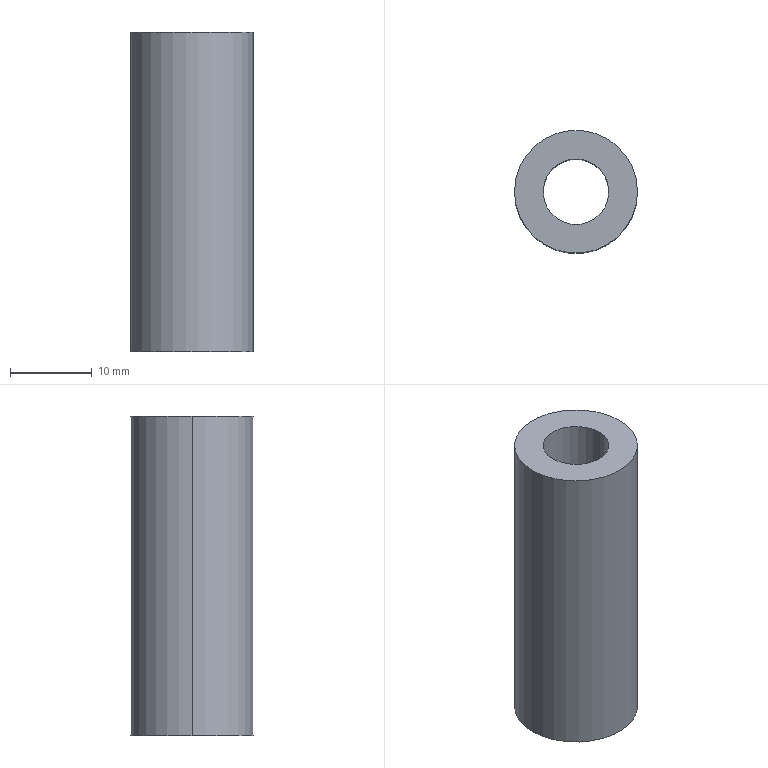Part | SolidWorks | features Extrusion 1 | 1 solid | 6 faces | box 15 x 15 x 39 mm | volume 4932 mm3 | cylinder 4 | plane 2 | commonest cylinder face diameters 8 x2 15 x2
STEP:
#1=CARTESIAN_POINT('',(-4.,0.,39.));
#2=VERTEX_POINT('',#1);
#3=CARTESIAN_POINT('',(4.,0.,39.));
#4=VERTEX_POINT('',#3);
#5=CARTESIAN_POINT('',(0.,0.,39.));
#6=DIRECTION('',(0.,0.,1.));
#7=DIRECTION('',(1.,0.,0.));
#8=AXIS2_PLACEMENT_3D('',#5,#6,#7);
#9=CIRCLE('',#8,4.);
#10=EDGE_CURVE('',#2,#4,#9,.T.);
#11=ORIENTED_EDGE('',*,*,#10,.T.);
#12=CARTESIAN_POINT('',(4.,0.,0.));
#13=VERTEX_POINT('',#12);
#14=CARTESIAN_POINT('',(4.,0.,39.));
#15=DIRECTION('',(0.,0.,-1.));
#16=VECTOR('',#15,1000.);
#17=LINE('',#14,#16);
#18=EDGE_CURVE('',#4,#13,#17,.T.);
#19=ORIENTED_EDGE('',*,*,#18,.T.);
#20=CARTESIAN_POINT('',(-4.,0.,0.));
#21=VERTEX_POINT('',#20);
#22=CARTESIAN_POINT('',(0.,0.,0.));
#23=DIRECTION('',(0.,0.,1.));
#24=DIRECTION('',(1.,0.,0.));
#25=AXIS2_PLACEMENT_3D('',#22,#23,#24);
#26=CIRCLE('',#25,4.);
#27=EDGE_CURVE('',#21,#13,#26,.T.);
#28=ORIENTED_EDGE('',*,*,#27,.F.);
#29=CARTESIAN_POINT('',(-4.,0.,39.));
#30=DIRECTION('',(0.,0.,-1.));
#31=VECTOR('',#30,1000.);
#32=LINE('',#29,#31);
#33=EDGE_CURVE('',#2,#21,#32,.T.);
#34=ORIENTED_EDGE('',*,*,#33,.F.);
#35=EDGE_LOOP('',(#11,#19,#28,#34));
#36=FACE_OUTER_BOUND('',#35,.T.);
#37=CARTESIAN_POINT('',(0.,0.,39.));
#38=DIRECTION('',(0.,0.,-1.));
#39=DIRECTION('',(-1.,0.,0.));
#40=AXIS2_PLACEMENT_3D('',#37,#38,#39);
#41=CYLINDRICAL_SURFACE('',#40,4.);
#42=ADVANCED_FACE('',(#36),#41,.F.);
#43=CARTESIAN_POINT('',(7.5,0.,39.));
#44=VERTEX_POINT('',#43);
#45=CARTESIAN_POINT('',(-7.5,0.,39.));
#46=VERTEX_POINT('',#45);
#47=CARTESIAN_POINT('',(0.,0.,39.));
#48=DIRECTION('',(0.,0.,1.));
#49=DIRECTION('',(1.,0.,0.));
#50=AXIS2_PLACEMENT_3D('',#47,#48,#49);
#51=CIRCLE('',#50,7.5);
#52=EDGE_CURVE('',#44,#46,#51,.T.);
#53=ORIENTED_EDGE('',*,*,#52,.F.);
#54=CARTESIAN_POINT('',(7.5,0.,0.));
#55=VERTEX_POINT('',#54);
#56=CARTESIAN_POINT('',(7.5,0.,39.));
#57=DIRECTION('',(0.,0.,-1.));
#58=VECTOR('',#57,1000.);
#59=LINE('',#56,#58);
#60=EDGE_CURVE('',#44,#55,#59,.T.);
#61=ORIENTED_EDGE('',*,*,#60,.T.);
#62=CARTESIAN_POINT('',(-7.5,0.,0.));
#63=VERTEX_POINT('',#62);
#64=CARTESIAN_POINT('',(0.,0.,0.));
#65=DIRECTION('',(0.,0.,1.));
#66=DIRECTION('',(1.,0.,0.));
#67=AXIS2_PLACEMENT_3D('',#64,#65,#66);
#68=CIRCLE('',#67,7.5);
#69=EDGE_CURVE('',#55,#63,#68,.T.);
#70=ORIENTED_EDGE('',*,*,#69,.T.);
#71=CARTESIAN_POINT('',(-7.5,0.,39.));
#72=DIRECTION('',(0.,0.,-1.));
#73=VECTOR('',#72,1000.);
#74=LINE('',#71,#73);
#75=EDGE_CURVE('',#46,#63,#74,.T.);
#76=ORIENTED_EDGE('',*,*,#75,.F.);
#77=EDGE_LOOP('',(#53,#61,#70,#76));
#78=FACE_OUTER_BOUND('',#77,.T.);
#79=CARTESIAN_POINT('',(0.,0.,39.));
#80=DIRECTION('',(0.,0.,-1.));
#81=DIRECTION('',(-1.,0.,0.));
#82=AXIS2_PLACEMENT_3D('',#79,#80,#81);
#83=CYLINDRICAL_SURFACE('',#82,7.5);
#84=ADVANCED_FACE('',(#78),#83,.T.);
#85=CARTESIAN_POINT('',(0.,0.,39.));
#86=DIRECTION('',(0.,0.,1.));
#87=DIRECTION('',(1.,0.,0.));
#88=AXIS2_PLACEMENT_3D('',#85,#86,#87);
#89=CIRCLE('',#88,7.5);
#90=EDGE_CURVE('',#46,#44,#89,.T.);
#91=ORIENTED_EDGE('',*,*,#90,.T.);
#92=ORIENTED_EDGE('',*,*,#52,.T.);
#93=EDGE_LOOP('',(#91,#92));
#94=FACE_OUTER_BOUND('',#93,.T.);
#95=ORIENTED_EDGE('',*,*,#10,.F.);
#96=CARTESIAN_POINT('',(0.,0.,39.));
#97=DIRECTION('',(0.,0.,1.));
#98=DIRECTION('',(1.,0.,0.));
#99=AXIS2_PLACEMENT_3D('',#96,#97,#98);
#100=CIRCLE('',#99,4.);
#101=EDGE_CURVE('',#4,#2,#100,.T.);
#102=ORIENTED_EDGE('',*,*,#101,.F.);
#103=EDGE_LOOP('',(#95,#102));
#104=FACE_BOUND('',#103,.T.);
#105=CARTESIAN_POINT('',(0.,0.,39.));
#106=DIRECTION('',(0.,0.,1.));
#107=DIRECTION('',(1.,0.,0.));
#108=AXIS2_PLACEMENT_3D('',#105,#106,#107);
#109=PLANE('',#108);
#110=ADVANCED_FACE('',(#94,#104),#109,.T.);
#111=CARTESIAN_POINT('',(0.,0.,0.));
#112=DIRECTION('',(0.,0.,1.));
#113=DIRECTION('',(1.,0.,0.));
#114=AXIS2_PLACEMENT_3D('',#111,#112,#113);
#115=CIRCLE('',#114,7.5);
#116=EDGE_CURVE('',#63,#55,#115,.T.);
#117=ORIENTED_EDGE('',*,*,#116,.F.);
#118=ORIENTED_EDGE('',*,*,#69,.F.);
#119=EDGE_LOOP('',(#117,#118));
#120=FACE_OUTER_BOUND('',#119,.T.);
#121=ORIENTED_EDGE('',*,*,#27,.T.);
#122=CARTESIAN_POINT('',(0.,0.,0.));
#123=DIRECTION('',(0.,0.,1.));
#124=DIRECTION('',(1.,0.,0.));
#125=AXIS2_PLACEMENT_3D('',#122,#123,#124);
#126=CIRCLE('',#125,4.);
#127=EDGE_CURVE('',#13,#21,#126,.T.);
#128=ORIENTED_EDGE('',*,*,#127,.T.);
#129=EDGE_LOOP('',(#121,#128));
#130=FACE_BOUND('',#129,.T.);
#131=CARTESIAN_POINT('',(0.,0.,0.));
#132=DIRECTION('',(0.,0.,1.));
#133=DIRECTION('',(1.,0.,0.));
#134=AXIS2_PLACEMENT_3D('',#131,#132,#133);
#135=PLANE('',#134);
#136=ADVANCED_FACE('',(#120,#130),#135,.F.);
#137=ORIENTED_EDGE('',*,*,#60,.F.);
#138=ORIENTED_EDGE('',*,*,#90,.F.);
#139=ORIENTED_EDGE('',*,*,#75,.T.);
#140=ORIENTED_EDGE('',*,*,#116,.T.);
#141=EDGE_LOOP('',(#137,#138,#139,#140));
#142=FACE_OUTER_BOUND('',#141,.T.);
#143=CARTESIAN_POINT('',(0.,0.,39.));
#144=DIRECTION('',(0.,0.,-1.));
#145=DIRECTION('',(-1.,0.,0.));
#146=AXIS2_PLACEMENT_3D('',#143,#144,#145);
#147=CYLINDRICAL_SURFACE('',#146,7.5);
#148=ADVANCED_FACE('',(#142),#147,.T.);
#149=ORIENTED_EDGE('',*,*,#18,.F.);
#150=ORIENTED_EDGE('',*,*,#101,.T.);
#151=ORIENTED_EDGE('',*,*,#33,.T.);
#152=ORIENTED_EDGE('',*,*,#127,.F.);
#153=EDGE_LOOP('',(#149,#150,#151,#152));
#154=FACE_OUTER_BOUND('',#153,.T.);
#155=CARTESIAN_POINT('',(0.,0.,39.));
#156=DIRECTION('',(0.,0.,-1.));
#157=DIRECTION('',(-1.,0.,0.));
#158=AXIS2_PLACEMENT_3D('',#155,#156,#157);
#159=CYLINDRICAL_SURFACE('',#158,4.);
#160=ADVANCED_FACE('',(#154),#159,.F.);
#161=CLOSED_SHELL('',(#42,#84,#110,#136,#148,#160));
#162=MANIFOLD_SOLID_BREP('',#161);
#163=CARTESIAN_POINT('',(0.,0.,0.));
#164=DIRECTION('',(0.,0.,1.));
#165=DIRECTION('',(1.,0.,0.));
#166=AXIS2_PLACEMENT_3D('',#163,#164,#165);
#167=(LENGTH_UNIT()NAMED_UNIT(*)SI_UNIT(.MILLI.,.METRE.));
#168=UNCERTAINTY_MEASURE_WITH_UNIT(LENGTH_MEASURE(0.00001),#167,'','');
#169=(NAMED_UNIT(*)PLANE_ANGLE_UNIT()SI_UNIT($,.RADIAN.));
#170=(NAMED_UNIT(*)SI_UNIT($,.STERADIAN.)SOLID_ANGLE_UNIT());
#171=(GEOMETRIC_REPRESENTATION_CONTEXT(3)GLOBAL_UNCERTAINTY_ASSIGNED_CONTEXT((#168))GLOBAL_UNIT_ASSIGNED_CONTEXT((#167,#169,#170))REPRESENTATION_CONTEXT('',''));
#172=ADVANCED_BREP_SHAPE_REPRESENTATION('',(#162,#166),#171);